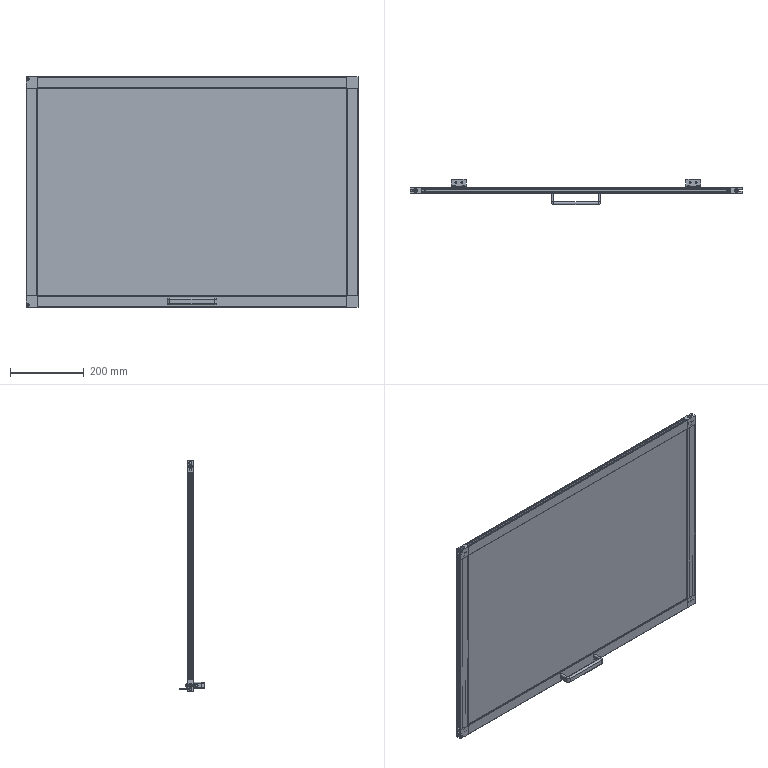Part | SolidWorks | features ReferencePattern 5, LocalLPattern 1 | 30 solids | 1032 faces | box 902 x 68 x 625 mm | volume 3235743 mm3 | plane 610 | cylinder 274 | cone 92 | spline 56 | commonest cylinder face diameters 5 x48 11 x48 4.5 x32 1 x24 3.3 x20 2 x16